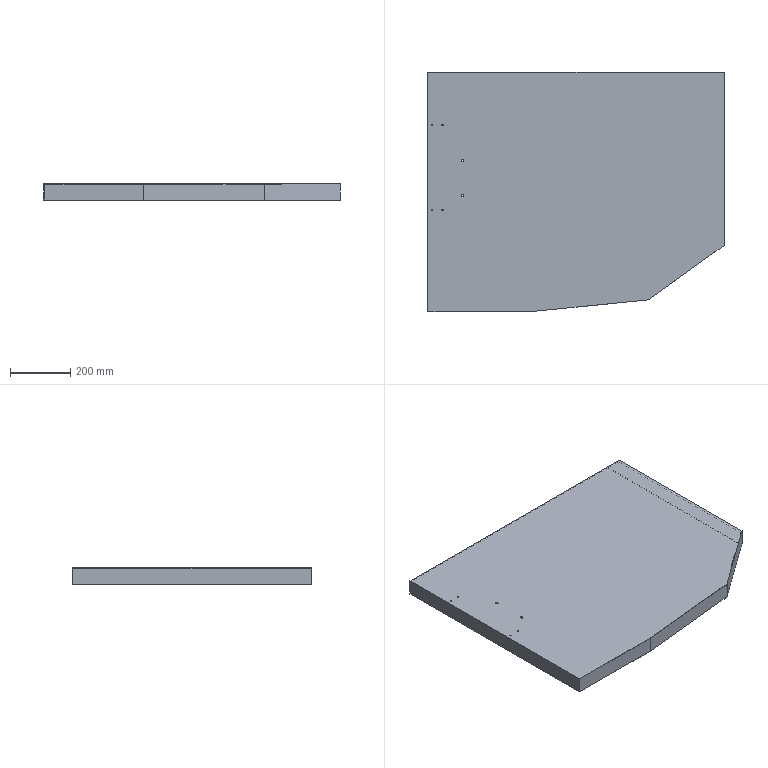Part | SolidWorks | features HoleWzd 2, ICE 2, BossThin 1, Cut 1, ExtruThin 1 | 1 solid | 41 faces | box 980 x 794 x 53 mm | volume 2935237 mm3 | plane 21 | cylinder 20 | commonest cylinder face diameters 4.2 x8 6.8 x8 8.2 x4
STEP:
#1=CARTESIAN_POINT('',(-417.615,-81.,50.));
#2=VERTEX_POINT('',#1);
#3=CARTESIAN_POINT('',(-413.415,-81.,50.));
#4=VERTEX_POINT('',#3);
#5=CARTESIAN_POINT('',(-415.515,-81.,50.));
#6=DIRECTION('',(0.,0.,1.));
#7=DIRECTION('',(1.,0.,0.));
#8=AXIS2_PLACEMENT_3D('',#5,#6,#7);
#9=CIRCLE('',#8,2.1);
#10=EDGE_CURVE('',#2,#4,#9,.T.);
#11=ORIENTED_EDGE('',*,*,#10,.F.);
#12=CARTESIAN_POINT('',(-417.615,-81.,53.));
#13=VERTEX_POINT('',#12);
#14=CARTESIAN_POINT('',(-417.615,-81.,53.));
#15=DIRECTION('',(0.,0.,1.));
#16=VECTOR('',#15,1000.);
#17=LINE('',#14,#16);
#18=EDGE_CURVE('',#2,#13,#17,.T.);
#19=ORIENTED_EDGE('',*,*,#18,.T.);
#20=CARTESIAN_POINT('',(-413.415,-81.,53.));
#21=VERTEX_POINT('',#20);
#22=CARTESIAN_POINT('',(-415.515,-81.,53.));
#23=DIRECTION('',(0.,0.,1.));
#24=DIRECTION('',(1.,0.,0.));
#25=AXIS2_PLACEMENT_3D('',#22,#23,#24);
#26=CIRCLE('',#25,2.1);
#27=EDGE_CURVE('',#13,#21,#26,.T.);
#28=ORIENTED_EDGE('',*,*,#27,.T.);
#29=CARTESIAN_POINT('',(-413.415,-81.,53.));
#30=DIRECTION('',(0.,0.,1.));
#31=VECTOR('',#30,1000.);
#32=LINE('',#29,#31);
#33=EDGE_CURVE('',#4,#21,#32,.T.);
#34=ORIENTED_EDGE('',*,*,#33,.F.);
#35=EDGE_LOOP('',(#11,#19,#28,#34));
#36=FACE_OUTER_BOUND('',#35,.T.);
#37=CARTESIAN_POINT('',(-415.515,-81.,53.));
#38=DIRECTION('',(0.,0.,1.));
#39=DIRECTION('',(1.,0.,0.));
#40=AXIS2_PLACEMENT_3D('',#37,#38,#39);
#41=CYLINDRICAL_SURFACE('',#40,2.1);
#42=ADVANCED_FACE('',(#36),#41,.F.);
#43=CARTESIAN_POINT('',(-384.115,-81.,50.));
#44=VERTEX_POINT('',#43);
#45=CARTESIAN_POINT('',(-379.915,-81.,50.));
#46=VERTEX_POINT('',#45);
#47=CARTESIAN_POINT('',(-382.015,-81.,50.));
#48=DIRECTION('',(0.,0.,1.));
#49=DIRECTION('',(1.,0.,0.));
#50=AXIS2_PLACEMENT_3D('',#47,#48,#49);
#51=CIRCLE('',#50,2.1);
#52=EDGE_CURVE('',#44,#46,#51,.T.);
#53=ORIENTED_EDGE('',*,*,#52,.F.);
#54=CARTESIAN_POINT('',(-384.115,-81.,53.));
#55=VERTEX_POINT('',#54);
#56=CARTESIAN_POINT('',(-384.115,-81.,53.));
#57=DIRECTION('',(0.,0.,1.));
#58=VECTOR('',#57,1000.);
#59=LINE('',#56,#58);
#60=EDGE_CURVE('',#44,#55,#59,.T.);
#61=ORIENTED_EDGE('',*,*,#60,.T.);
#62=CARTESIAN_POINT('',(-379.915,-81.,53.));
#63=VERTEX_POINT('',#62);
#64=CARTESIAN_POINT('',(-382.015,-81.,53.));
#65=DIRECTION('',(0.,0.,1.));
#66=DIRECTION('',(1.,0.,0.));
#67=AXIS2_PLACEMENT_3D('',#64,#65,#66);
#68=CIRCLE('',#67,2.1);
#69=EDGE_CURVE('',#55,#63,#68,.T.);
#70=ORIENTED_EDGE('',*,*,#69,.T.);
#71=CARTESIAN_POINT('',(-379.915,-81.,53.));
#72=DIRECTION('',(0.,0.,1.));
#73=VECTOR('',#72,1000.);
#74=LINE('',#71,#73);
#75=EDGE_CURVE('',#46,#63,#74,.T.);
#76=ORIENTED_EDGE('',*,*,#75,.F.);
#77=EDGE_LOOP('',(#53,#61,#70,#76));
#78=FACE_OUTER_BOUND('',#77,.T.);
#79=CARTESIAN_POINT('',(-382.015,-81.,53.));
#80=DIRECTION('',(0.,0.,1.));
#81=DIRECTION('',(1.,0.,0.));
#82=AXIS2_PLACEMENT_3D('',#79,#80,#81);
#83=CYLINDRICAL_SURFACE('',#82,2.1);
#84=ADVANCED_FACE('',(#78),#83,.F.);
#85=CARTESIAN_POINT('',(-417.615,199.,50.));
#86=VERTEX_POINT('',#85);
#87=CARTESIAN_POINT('',(-413.415,199.,50.));
#88=VERTEX_POINT('',#87);
#89=CARTESIAN_POINT('',(-415.515,199.,50.));
#90=DIRECTION('',(0.,0.,1.));
#91=DIRECTION('',(1.,0.,0.));
#92=AXIS2_PLACEMENT_3D('',#89,#90,#91);
#93=CIRCLE('',#92,2.1);
#94=EDGE_CURVE('',#86,#88,#93,.T.);
#95=ORIENTED_EDGE('',*,*,#94,.F.);
#96=CARTESIAN_POINT('',(-417.615,199.,53.));
#97=VERTEX_POINT('',#96);
#98=CARTESIAN_POINT('',(-417.615,199.,53.));
#99=DIRECTION('',(0.,0.,1.));
#100=VECTOR('',#99,1000.);
#101=LINE('',#98,#100);
#102=EDGE_CURVE('',#86,#97,#101,.T.);
#103=ORIENTED_EDGE('',*,*,#102,.T.);
#104=CARTESIAN_POINT('',(-413.415,199.,53.));
#105=VERTEX_POINT('',#104);
#106=CARTESIAN_POINT('',(-415.515,199.,53.));
#107=DIRECTION('',(0.,0.,1.));
#108=DIRECTION('',(1.,0.,0.));
#109=AXIS2_PLACEMENT_3D('',#106,#107,#108);
#110=CIRCLE('',#109,2.1);
#111=EDGE_CURVE('',#97,#105,#110,.T.);
#112=ORIENTED_EDGE('',*,*,#111,.T.);
#113=CARTESIAN_POINT('',(-413.415,199.,53.));
#114=DIRECTION('',(0.,0.,1.));
#115=VECTOR('',#114,1000.);
#116=LINE('',#113,#115);
#117=EDGE_CURVE('',#88,#105,#116,.T.);
#118=ORIENTED_EDGE('',*,*,#117,.F.);
#119=EDGE_LOOP('',(#95,#103,#112,#118));
#120=FACE_OUTER_BOUND('',#119,.T.);
#121=CARTESIAN_POINT('',(-415.515,199.,53.));
#122=DIRECTION('',(0.,0.,1.));
#123=DIRECTION('',(1.,0.,0.));
#124=AXIS2_PLACEMENT_3D('',#121,#122,#123);
#125=CYLINDRICAL_SURFACE('',#124,2.1);
#126=ADVANCED_FACE('',(#120),#125,.F.);
#127=CARTESIAN_POINT('',(-384.115,199.,50.));
#128=VERTEX_POINT('',#127);
#129=CARTESIAN_POINT('',(-379.915,199.,50.));
#130=VERTEX_POINT('',#129);
#131=CARTESIAN_POINT('',(-382.015,199.,50.));
#132=DIRECTION('',(0.,0.,1.));
#133=DIRECTION('',(1.,0.,0.));
#134=AXIS2_PLACEMENT_3D('',#131,#132,#133);
#135=CIRCLE('',#134,2.1);
#136=EDGE_CURVE('',#128,#130,#135,.T.);
#137=ORIENTED_EDGE('',*,*,#136,.F.);
#138=CARTESIAN_POINT('',(-384.115,199.,53.));
#139=VERTEX_POINT('',#138);
#140=CARTESIAN_POINT('',(-384.115,199.,53.));
#141=DIRECTION('',(0.,0.,1.));
#142=VECTOR('',#141,1000.);
#143=LINE('',#140,#142);
#144=EDGE_CURVE('',#128,#139,#143,.T.);
#145=ORIENTED_EDGE('',*,*,#144,.T.);
#146=CARTESIAN_POINT('',(-379.915,199.,53.));
#147=VERTEX_POINT('',#146);
#148=CARTESIAN_POINT('',(-382.015,199.,53.));
#149=DIRECTION('',(0.,0.,1.));
#150=DIRECTION('',(1.,0.,0.));
#151=AXIS2_PLACEMENT_3D('',#148,#149,#150);
#152=CIRCLE('',#151,2.1);
#153=EDGE_CURVE('',#139,#147,#152,.T.);
#154=ORIENTED_EDGE('',*,*,#153,.T.);
#155=CARTESIAN_POINT('',(-379.915,199.,53.));
#156=DIRECTION('',(0.,0.,1.));
#157=VECTOR('',#156,1000.);
#158=LINE('',#155,#157);
#159=EDGE_CURVE('',#130,#147,#158,.T.);
#160=ORIENTED_EDGE('',*,*,#159,.F.);
#161=EDGE_LOOP('',(#137,#145,#154,#160));
#162=FACE_OUTER_BOUND('',#161,.T.);
#163=CARTESIAN_POINT('',(-382.015,199.,53.));
#164=DIRECTION('',(0.,0.,1.));
#165=DIRECTION('',(1.,0.,0.));
#166=AXIS2_PLACEMENT_3D('',#163,#164,#165);
#167=CYLINDRICAL_SURFACE('',#166,2.1);
#168=ADVANCED_FACE('',(#162),#167,.F.);
#169=CARTESIAN_POINT('',(542.,315.,24.4));
#170=VERTEX_POINT('',#169);
#171=CARTESIAN_POINT('',(542.,315.,17.6));
#172=VERTEX_POINT('',#171);
#173=CARTESIAN_POINT('',(542.,315.,21.));
#174=DIRECTION('',(1.,0.,0.));
#175=DIRECTION('',(0.,0.,-1.));
#176=AXIS2_PLACEMENT_3D('',#173,#174,#175);
#177=CIRCLE('',#176,3.4);
#178=EDGE_CURVE('',#170,#172,#177,.T.);
#179=ORIENTED_EDGE('',*,*,#178,.F.);
#180=CARTESIAN_POINT('',(550.,315.,24.4));
#181=VERTEX_POINT('',#180);
#182=CARTESIAN_POINT('',(550.,315.,24.4));
#183=DIRECTION('',(1.,0.,0.));
#184=VECTOR('',#183,1000.);
#185=LINE('',#182,#184);
#186=EDGE_CURVE('',#170,#181,#185,.T.);
#187=ORIENTED_EDGE('',*,*,#186,.T.);
#188=CARTESIAN_POINT('',(550.,315.,17.6));
#189=VERTEX_POINT('',#188);
#190=CARTESIAN_POINT('',(550.,315.,21.));
#191=DIRECTION('',(1.,0.,0.));
#192=DIRECTION('',(0.,0.,-1.));
#193=AXIS2_PLACEMENT_3D('',#190,#191,#192);
#194=CIRCLE('',#193,3.4);
#195=EDGE_CURVE('',#181,#189,#194,.T.);
#196=ORIENTED_EDGE('',*,*,#195,.T.);
#197=CARTESIAN_POINT('',(550.,315.,17.6));
#198=DIRECTION('',(1.,0.,0.));
#199=VECTOR('',#198,1000.);
#200=LINE('',#197,#199);
#201=EDGE_CURVE('',#172,#189,#200,.T.);
#202=ORIENTED_EDGE('',*,*,#201,.F.);
#203=EDGE_LOOP('',(#179,#187,#196,#202));
#204=FACE_OUTER_BOUND('',#203,.T.);
#205=CARTESIAN_POINT('',(550.,315.,21.));
#206=DIRECTION('',(1.,0.,0.));
#207=DIRECTION('',(0.,0.,-1.));
#208=AXIS2_PLACEMENT_3D('',#205,#206,#207);
#209=CYLINDRICAL_SURFACE('',#208,3.4);
#210=ADVANCED_FACE('',(#204),#209,.F.);
#211=CARTESIAN_POINT('',(542.,285.,24.4));
#212=VERTEX_POINT('',#211);
#213=CARTESIAN_POINT('',(542.,285.,17.6));
#214=VERTEX_POINT('',#213);
#215=CARTESIAN_POINT('',(542.,285.,21.));
#216=DIRECTION('',(1.,0.,0.));
#217=DIRECTION('',(0.,0.,-1.));
#218=AXIS2_PLACEMENT_3D('',#215,#216,#217);
#219=CIRCLE('',#218,3.4);
#220=EDGE_CURVE('',#212,#214,#219,.T.);
#221=ORIENTED_EDGE('',*,*,#220,.F.);
#222=CARTESIAN_POINT('',(550.,285.,24.4));
#223=VERTEX_POINT('',#222);
#224=CARTESIAN_POINT('',(550.,285.,24.4));
#225=DIRECTION('',(1.,0.,0.));
#226=VECTOR('',#225,1000.);
#227=LINE('',#224,#226);
#228=EDGE_CURVE('',#212,#223,#227,.T.);
#229=ORIENTED_EDGE('',*,*,#228,.T.);
#230=CARTESIAN_POINT('',(550.,285.,17.6));
#231=VERTEX_POINT('',#230);
#232=CARTESIAN_POINT('',(550.,285.,21.));
#233=DIRECTION('',(1.,0.,0.));
#234=DIRECTION('',(0.,0.,-1.));
#235=AXIS2_PLACEMENT_3D('',#232,#233,#234);
#236=CIRCLE('',#235,3.4);
#237=EDGE_CURVE('',#223,#231,#236,.T.);
#238=ORIENTED_EDGE('',*,*,#237,.T.);
#239=CARTESIAN_POINT('',(550.,285.,17.6));
#240=DIRECTION('',(1.,0.,0.));
#241=VECTOR('',#240,1000.);
#242=LINE('',#239,#241);
#243=EDGE_CURVE('',#214,#231,#242,.T.);
#244=ORIENTED_EDGE('',*,*,#243,.F.);
#245=EDGE_LOOP('',(#221,#229,#238,#244));
#246=FACE_OUTER_BOUND('',#245,.T.);
#247=CARTESIAN_POINT('',(550.,285.,21.));
#248=DIRECTION('',(1.,0.,0.));
#249=DIRECTION('',(0.,0.,-1.));
#250=AXIS2_PLACEMENT_3D('',#247,#248,#249);
#251=CYLINDRICAL_SURFACE('',#250,3.4);
#252=ADVANCED_FACE('',(#246),#251,.F.);
#253=CARTESIAN_POINT('',(542.,45.,24.4));
#254=VERTEX_POINT('',#253);
#255=CARTESIAN_POINT('',(542.,45.,17.6));
#256=VERTEX_POINT('',#255);
#257=CARTESIAN_POINT('',(542.,45.,21.));
#258=DIRECTION('',(1.,0.,0.));
#259=DIRECTION('',(0.,0.,-1.));
#260=AXIS2_PLACEMENT_3D('',#257,#258,#259);
#261=CIRCLE('',#260,3.4);
#262=EDGE_CURVE('',#254,#256,#261,.T.);
#263=ORIENTED_EDGE('',*,*,#262,.F.);
#264=CARTESIAN_POINT('',(550.,45.,24.4));
#265=VERTEX_POINT('',#264);
#266=CARTESIAN_POINT('',(550.,45.,24.4));
#267=DIRECTION('',(1.,0.,0.));
#268=VECTOR('',#267,1000.);
#269=LINE('',#266,#268);
#270=EDGE_CURVE('',#254,#265,#269,.T.);
#271=ORIENTED_EDGE('',*,*,#270,.T.);
#272=CARTESIAN_POINT('',(550.,45.,17.6));
#273=VERTEX_POINT('',#272);
#274=CARTESIAN_POINT('',(550.,45.,21.));
#275=DIRECTION('',(1.,0.,0.));
#276=DIRECTION('',(0.,0.,-1.));
#277=AXIS2_PLACEMENT_3D('',#274,#275,#276);
#278=CIRCLE('',#277,3.4);
#279=EDGE_CURVE('',#265,#273,#278,.T.);
#280=ORIENTED_EDGE('',*,*,#279,.T.);
#281=CARTESIAN_POINT('',(550.,45.,17.6));
#282=DIRECTION('',(1.,0.,0.));
#283=VECTOR('',#282,1000.);
#284=LINE('',#281,#283);
#285=EDGE_CURVE('',#256,#273,#284,.T.);
#286=ORIENTED_EDGE('',*,*,#285,.F.);
#287=EDGE_LOOP('',(#263,#271,#280,#286));
#288=FACE_OUTER_BOUND('',#287,.T.);
#289=CARTESIAN_POINT('',(550.,45.,21.));
#290=DIRECTION('',(1.,0.,0.));
#291=DIRECTION('',(0.,0.,-1.));
#292=AXIS2_PLACEMENT_3D('',#289,#290,#291);
#293=CYLINDRICAL_SURFACE('',#292,3.4);
#294=ADVANCED_FACE('',(#288),#293,.F.);
#295=CARTESIAN_POINT('',(-312.4,82.25,50.));
#296=VERTEX_POINT('',#295);
#297=CARTESIAN_POINT('',(-320.6,82.25,50.));
#298=VERTEX_POINT('',#297);
#299=CARTESIAN_POINT('',(-316.5,82.25,50.));
#300=DIRECTION('',(0.,0.,-1.));
#301=DIRECTION('',(1.,0.,0.));
#302=AXIS2_PLACEMENT_3D('',#299,#300,#301);
#303=CIRCLE('',#302,4.1);
#304=EDGE_CURVE('',#296,#298,#303,.T.);
#305=ORIENTED_EDGE('',*,*,#304,.T.);
#306=CARTESIAN_POINT('',(-320.6,82.25,53.));
#307=VERTEX_POINT('',#306);
#308=CARTESIAN_POINT('',(-320.6,82.25,-0.001));
#309=DIRECTION('',(0.,0.,1.));
#310=VECTOR('',#309,1000.);
#311=LINE('',#308,#310);
#312=EDGE_CURVE('',#298,#307,#311,.T.);
#313=ORIENTED_EDGE('',*,*,#312,.T.);
#314=CARTESIAN_POINT('',(-312.4,82.25,53.));
#315=VERTEX_POINT('',#314);
#316=CARTESIAN_POINT('',(-316.5,82.25,53.));
#317=DIRECTION('',(0.,0.,1.));
#318=DIRECTION('',(1.,0.,0.));
#319=AXIS2_PLACEMENT_3D('',#316,#317,#318);
#320=CIRCLE('',#319,4.1);
#321=EDGE_CURVE('',#307,#315,#320,.T.);
#322=ORIENTED_EDGE('',*,*,#321,.T.);
#323=CARTESIAN_POINT('',(-312.4,82.25,-0.001));
#324=DIRECTION('',(0.,0.,1.));
#325=VECTOR('',#324,1000.);
#326=LINE('',#323,#325);
#327=EDGE_CURVE('',#296,#315,#326,.T.);
#328=ORIENTED_EDGE('',*,*,#327,.F.);
#329=EDGE_LOOP('',(#305,#313,#322,#328));
#330=FACE_OUTER_BOUND('',#329,.T.);
#331=CARTESIAN_POINT('',(-316.5,82.25,-0.001));
#332=DIRECTION('',(0.,0.,1.));
#333=DIRECTION('',(1.,0.,0.));
#334=AXIS2_PLACEMENT_3D('',#331,#332,#333);
#335=CYLINDRICAL_SURFACE('',#334,4.1);
#336=ADVANCED_FACE('',(#330),#335,.F.);
#337=CARTESIAN_POINT('',(-312.4,-34.25,50.));
#338=VERTEX_POINT('',#337);
#339=CARTESIAN_POINT('',(-320.6,-34.25,50.));
#340=VERTEX_POINT('',#339);
#341=CARTESIAN_POINT('',(-316.5,-34.25,50.));
#342=DIRECTION('',(0.,0.,-1.));
#343=DIRECTION('',(1.,0.,0.));
#344=AXIS2_PLACEMENT_3D('',#341,#342,#343);
#345=CIRCLE('',#344,4.1);
#346=EDGE_CURVE('',#338,#340,#345,.T.);
#347=ORIENTED_EDGE('',*,*,#346,.T.);
#348=CARTESIAN_POINT('',(-320.6,-34.25,53.));
#349=VERTEX_POINT('',#348);
#350=CARTESIAN_POINT('',(-320.6,-34.25,-0.001));
#351=DIRECTION('',(0.,0.,1.));
#352=VECTOR('',#351,1000.);
#353=LINE('',#350,#352);
#354=EDGE_CURVE('',#340,#349,#353,.T.);
#355=ORIENTED_EDGE('',*,*,#354,.T.);
#356=CARTESIAN_POINT('',(-312.4,-34.25,53.));
#357=VERTEX_POINT('',#356);
#358=CARTESIAN_POINT('',(-316.5,-34.25,53.));
#359=DIRECTION('',(0.,0.,1.));
#360=DIRECTION('',(1.,0.,0.));
#361=AXIS2_PLACEMENT_3D('',#358,#359,#360);
#362=CIRCLE('',#361,4.1);
#363=EDGE_CURVE('',#349,#357,#362,.T.);
#364=ORIENTED_EDGE('',*,*,#363,.T.);
#365=CARTESIAN_POINT('',(-312.4,-34.25,-0.001));
#366=DIRECTION('',(0.,0.,1.));
#367=VECTOR('',#366,1000.);
#368=LINE('',#365,#367);
#369=EDGE_CURVE('',#338,#357,#368,.T.);
#370=ORIENTED_EDGE('',*,*,#369,.F.);
#371=EDGE_LOOP('',(#347,#355,#364,#370));
#372=FACE_OUTER_BOUND('',#371,.T.);
#373=CARTESIAN_POINT('',(-316.5,-34.25,-0.001));
#374=DIRECTION('',(0.,0.,1.));
#375=DIRECTION('',(1.,0.,0.));
#376=AXIS2_PLACEMENT_3D('',#373,#374,#375);
#377=CYLINDRICAL_SURFACE('',#376,4.1);
#378=ADVANCED_FACE('',(#372),#377,.F.);
#379=CARTESIAN_POINT('',(542.,15.,24.4));
#380=VERTEX_POINT('',#379);
#381=CARTESIAN_POINT('',(542.,15.,17.6));
#382=VERTEX_POINT('',#381);
#383=CARTESIAN_POINT('',(542.,15.,21.));
#384=DIRECTION('',(1.,0.,0.));
#385=DIRECTION('',(0.,0.,-1.));
#386=AXIS2_PLACEMENT_3D('',#383,#384,#385);
#387=CIRCLE('',#386,3.4);
#388=EDGE_CURVE('',#380,#382,#387,.T.);
#389=ORIENTED_EDGE('',*,*,#388,.F.);
#390=CARTESIAN_POINT('',(550.,15.,24.4));
#391=VERTEX_POINT('',#390);
#392=CARTESIAN_POINT('',(550.,15.,24.4));
#393=DIRECTION('',(1.,0.,0.));
#394=VECTOR('',#393,1000.);
#395=LINE('',#392,#394);
#396=EDGE_CURVE('',#380,#391,#395,.T.);
#397=ORIENTED_EDGE('',*,*,#396,.T.);
#398=CARTESIAN_POINT('',(550.,15.,17.6));
#399=VERTEX_POINT('',#398);
#400=CARTESIAN_POINT('',(550.,15.,21.));
#401=DIRECTION('',(1.,0.,0.));
#402=DIRECTION('',(0.,0.,-1.));
#403=AXIS2_PLACEMENT_3D('',#400,#401,#402);
#404=CIRCLE('',#403,3.4);
#405=EDGE_CURVE('',#391,#399,#404,.T.);
#406=ORIENTED_EDGE('',*,*,#405,.T.);
#407=CARTESIAN_POINT('',(550.,15.,17.6));
#408=DIRECTION('',(1.,0.,0.));
#409=VECTOR('',#408,1000.);
#410=LINE('',#407,#409);
#411=EDGE_CURVE('',#382,#399,#410,.T.);
#412=ORIENTED_EDGE('',*,*,#411,.F.);
#413=EDGE_LOOP('',(#389,#397,#406,#412));
#414=FACE_OUTER_BOUND('',#413,.T.);
#415=CARTESIAN_POINT('',(550.,15.,21.));
#416=DIRECTION('',(1.,0.,0.));
#417=DIRECTION('',(0.,0.,-1.));
#418=AXIS2_PLACEMENT_3D('',#415,#416,#417);
#419=CYLINDRICAL_SURFACE('',#418,3.4);
#420=ADVANCED_FACE('',(#414),#419,.F.);
#421=CARTESIAN_POINT('',(550.,-199.,53.));
#422=VERTEX_POINT('',#421);
#423=CARTESIAN_POINT('',(550.,-199.,0.));
#424=VERTEX_POINT('',#423);
#425=CARTESIAN_POINT('',(550.,-199.,53.));
#426=DIRECTION('',(0.,0.,-1.));
#427=VECTOR('',#426,1000.);
#428=LINE('',#425,#427);
#429=EDGE_CURVE('',#422,#424,#428,.T.);
#430=ORIENTED_EDGE('',*,*,#429,.T.);
#431=CARTESIAN_POINT('',(550.,375.,0.));
#432=VERTEX_POINT('',#431);
#433=CARTESIAN_POINT('',(550.,375.,0.));
#434=DIRECTION('',(0.,1.,0.));
#435=VECTOR('',#434,1000.);
#436=LINE('',#433,#435);
#437=EDGE_CURVE('',#424,#432,#436,.T.);
#438=ORIENTED_EDGE('',*,*,#437,.T.);
#439=CARTESIAN_POINT('',(550.,375.,53.));
#440=VERTEX_POINT('',#439);
#441=CARTESIAN_POINT('',(550.,375.,53.));
#442=DIRECTION('',(0.,0.,-1.));
#443=VECTOR('',#442,1000.);
#444=LINE('',#441,#443);
#445=EDGE_CURVE('',#440,#432,#444,.T.);
#446=ORIENTED_EDGE('',*,*,#445,.F.);
#447=CARTESIAN_POINT('',(550.,375.,53.));
#448=DIRECTION('',(0.,1.,0.));
#449=VECTOR('',#448,1000.);
#450=LINE('',#447,#449);
#451=EDGE_CURVE('',#422,#440,#450,.T.);
#452=ORIENTED_EDGE('',*,*,#451,.F.);
#453=EDGE_LOOP('',(#430,#438,#446,#452));
#454=FACE_OUTER_BOUND('',#453,.T.);
#455=CARTESIAN_POINT('',(550.,15.,21.));
#456=DIRECTION('',(1.,0.,0.));
#457=DIRECTION('',(0.,0.,-1.));
#458=AXIS2_PLACEMENT_3D('',#455,#456,#457);
#459=CIRCLE('',#458,3.4);
#460=EDGE_CURVE('',#399,#391,#459,.T.);
#461=ORIENTED_EDGE('',*,*,#460,.F.);
#462=ORIENTED_EDGE('',*,*,#405,.F.);
#463=EDGE_LOOP('',(#461,#462));
#464=FACE_BOUND('',#463,.T.);
#465=CARTESIAN_POINT('',(550.,45.,21.));
#466=DIRECTION('',(1.,0.,0.));
#467=DIRECTION('',(0.,0.,-1.));
#468=AXIS2_PLACEMENT_3D('',#465,#466,#467);
#469=CIRCLE('',#468,3.4);
#470=EDGE_CURVE('',#273,#265,#469,.T.);
#471=ORIENTED_EDGE('',*,*,#470,.F.);
#472=ORIENTED_EDGE('',*,*,#279,.F.);
#473=EDGE_LOOP('',(#471,#472));
#474=FACE_BOUND('',#473,.T.);
#475=CARTESIAN_POINT('',(550.,285.,21.));
#476=DIRECTION('',(1.,0.,0.));
#477=DIRECTION('',(0.,0.,-1.));
#478=AXIS2_PLACEMENT_3D('',#475,#476,#477);
#479=CIRCLE('',#478,3.4);
#480=EDGE_CURVE('',#231,#223,#479,.T.);
#481=ORIENTED_EDGE('',*,*,#480,.F.);
#482=ORIENTED_EDGE('',*,*,#237,.F.);
#483=EDGE_LOOP('',(#481,#482));
#484=FACE_BOUND('',#483,.T.);
#485=CARTESIAN_POINT('',(550.,315.,21.));
#486=DIRECTION('',(1.,0.,0.));
#487=DIRECTION('',(0.,0.,-1.));
#488=AXIS2_PLACEMENT_3D('',#485,#486,#487);
#489=CIRCLE('',#488,3.4);
#490=EDGE_CURVE('',#189,#181,#489,.T.);
#491=ORIENTED_EDGE('',*,*,#490,.F.);
#492=ORIENTED_EDGE('',*,*,#195,.F.);
#493=EDGE_LOOP('',(#491,#492));
#494=FACE_BOUND('',#493,.T.);
#495=CARTESIAN_POINT('',(550.,375.,53.));
#496=DIRECTION('',(-1.,0.,0.));
#497=DIRECTION('',(0.,-1.,0.));
#498=AXIS2_PLACEMENT_3D('',#495,#496,#497);
#499=PLANE('',#498);
#500=ADVANCED_FACE('',(#454,#464,#474,#484,#494),#499,.F.);
#501=CARTESIAN_POINT('',(542.,315.,21.));
#502=DIRECTION('',(1.,0.,0.));
#503=DIRECTION('',(0.,0.,-1.));
#504=AXIS2_PLACEMENT_3D('',#501,#502,#503);
#505=CIRCLE('',#504,3.4);
#506=EDGE_CURVE('',#172,#170,#505,.T.);
#507=ORIENTED_EDGE('',*,*,#506,.T.);
#508=ORIENTED_EDGE('',*,*,#178,.T.);
#509=EDGE_LOOP('',(#507,#508));
#510=FACE_BOUND('',#509,.T.);
#511=CARTESIAN_POINT('',(542.,285.,21.));
#512=DIRECTION('',(1.,0.,0.));
#513=DIRECTION('',(0.,0.,-1.));
#514=AXIS2_PLACEMENT_3D('',#511,#512,#513);
#515=CIRCLE('',#514,3.4);
#516=EDGE_CURVE('',#214,#212,#515,.T.);
#517=ORIENTED_EDGE('',*,*,#516,.T.);
#518=ORIENTED_EDGE('',*,*,#220,.T.);
#519=EDGE_LOOP('',(#517,#518));
#520=FACE_BOUND('',#519,.T.);
#521=CARTESIAN_POINT('',(542.,45.,21.));
#522=DIRECTION('',(1.,0.,0.));
#523=DIRECTION('',(0.,0.,-1.));
#524=AXIS2_PLACEMENT_3D('',#521,#522,#523);
#525=CIRCLE('',#524,3.4);
#526=EDGE_CURVE('',#256,#254,#525,.T.);
#527=ORIENTED_EDGE('',*,*,#526,.T.);
#528=ORIENTED_EDGE('',*,*,#262,.T.);
#529=EDGE_LOOP('',(#527,#528));
#530=FACE_BOUND('',#529,.T.);
#531=CARTESIAN_POINT('',(542.,15.,21.));
#532=DIRECTION('',(1.,0.,0.));
#533=DIRECTION('',(0.,0.,-1.));
#534=AXIS2_PLACEMENT_3D('',#531,#532,#533);
#535=CIRCLE('',#534,3.4);
#536=EDGE_CURVE('',#382,#380,#535,.T.);
#537=ORIENTED_EDGE('',*,*,#536,.T.);
#538=ORIENTED_EDGE('',*,*,#388,.T.);
#539=EDGE_LOOP('',(#537,#538));
#540=FACE_BOUND('',#539,.T.);
#541=CARTESIAN_POINT('',(542.,372.,10.612));
#542=VERTEX_POINT('',#541);
#543=CARTESIAN_POINT('',(542.,372.,50.));
#544=VERTEX_POINT('',#543);
#545=CARTESIAN_POINT('',(542.,372.,53.));
#546=DIRECTION('',(0.,0.,1.));
#547=VECTOR('',#546,1000.);
#548=LINE('',#545,#547);
#549=EDGE_CURVE('',#542,#544,#548,.T.);
#550=ORIENTED_EDGE('',*,*,#549,.F.);
#551=CARTESIAN_POINT('',(542.,-201.063,10.612));
#552=VERTEX_POINT('',#551);
#553=CARTESIAN_POINT('',(542.,-201.063,10.612));
#554=DIRECTION('',(0.,-1.,0.));
#555=VECTOR('',#554,1000.);
#556=LINE('',#553,#555);
#557=EDGE_CURVE('',#542,#552,#556,.T.);
#558=ORIENTED_EDGE('',*,*,#557,.T.);
#559=CARTESIAN_POINT('',(542.,-201.063,50.));
#560=VERTEX_POINT('',#559);
#561=CARTESIAN_POINT('',(542.,-201.063,-576.119));
#562=DIRECTION('',(0.,0.,1.));
#563=VECTOR('',#562,1000.);
#564=LINE('',#561,#563);
#565=EDGE_CURVE('',#552,#560,#564,.T.);
#566=ORIENTED_EDGE('',*,*,#565,.T.);
#567=CARTESIAN_POINT('',(542.,-201.063,50.));
#568=DIRECTION('',(0.,1.,0.));
#569=VECTOR('',#568,1000.);
#570=LINE('',#567,#569);
#571=EDGE_CURVE('',#560,#544,#570,.T.);
#572=ORIENTED_EDGE('',*,*,#571,.T.);
#573=EDGE_LOOP('',(#550,#558,#566,#572));
#574=FACE_OUTER_BOUND('',#573,.T.);
#575=CARTESIAN_POINT('',(542.,-201.063,-576.119));
#576=DIRECTION('',(1.,0.,0.));
#577=DIRECTION('',(0.,0.,-1.));
#578=AXIS2_PLACEMENT_3D('',#575,#576,#577);
#579=PLANE('',#578);
#580=ADVANCED_FACE('',(#510,#520,#530,#540,#574),#579,.F.);
#581=CARTESIAN_POINT('',(495.109,-234.824,50.));
#582=VERTEX_POINT('',#581);
#583=CARTESIAN_POINT('',(280.386,-389.425,50.));
#584=DIRECTION('',(0.8115,0.5843,0.));
#585=VECTOR('',#584,1000.);
#586=LINE('',#583,#585);
#587=EDGE_CURVE('',#582,#560,#586,.T.);
#588=ORIENTED_EDGE('',*,*,#587,.F.);
#589=CARTESIAN_POINT('',(495.109,372.,50.));
#590=VERTEX_POINT('',#589);
#591=CARTESIAN_POINT('',(495.109,0.,50.));
#592=DIRECTION('',(0.,1.,0.));
#593=VECTOR('',#592,1000.);
#594=LINE('',#591,#593);
#595=EDGE_CURVE('',#582,#590,#594,.T.);
#596=ORIENTED_EDGE('',*,*,#595,.T.);
#597=CARTESIAN_POINT('',(0.,372.,50.));
#598=DIRECTION('',(-1.,0.,0.));
#599=VECTOR('',#598,1000.);
#600=LINE('',#597,#599);
#601=EDGE_CURVE('',#544,#590,#600,.T.);
#602=ORIENTED_EDGE('',*,*,#601,.F.);
#603=ORIENTED_EDGE('',*,*,#571,.F.);
#604=EDGE_LOOP('',(#588,#596,#602,#603));
#605=FACE_OUTER_BOUND('',#604,.T.);
#606=CARTESIAN_POINT('',(0.,0.,50.));
#607=DIRECTION('',(0.,0.,1.));
#608=DIRECTION('',(1.,0.,0.));
#609=AXIS2_PLACEMENT_3D('',#606,#607,#608);
#610=PLANE('',#609);
#611=ADVANCED_FACE('',(#605),#610,.F.);
#612=CARTESIAN_POINT('',(474.657,-249.55,67.18));
#613=DIRECTION('',(-0.6706,-0.4828,0.5633));
#614=VECTOR('',#613,1000.);
#615=LINE('',#612,#614);
#616=EDGE_CURVE('',#552,#582,#615,.T.);
#617=ORIENTED_EDGE('',*,*,#616,.T.);
#618=ORIENTED_EDGE('',*,*,#587,.T.);
#619=ORIENTED_EDGE('',*,*,#565,.F.);
#620=EDGE_LOOP('',(#617,#618,#619));
#621=FACE_OUTER_BOUND('',#620,.T.);
#622=CARTESIAN_POINT('',(280.386,-389.425,53.));
#623=DIRECTION('',(-0.5843,0.8115,0.));
#624=DIRECTION('',(-0.8115,-0.5843,0.));
#625=AXIS2_PLACEMENT_3D('',#622,#623,#624);
#626=PLANE('',#625);
#627=ADVANCED_FACE('',(#621),#626,.T.);
#628=CARTESIAN_POINT('',(493.286,372.,51.531));
#629=DIRECTION('',(0.7657,0.,-0.6432));
#630=VECTOR('',#629,1000.);
#631=LINE('',#628,#630);
#632=EDGE_CURVE('',#590,#542,#631,.T.);
#633=ORIENTED_EDGE('',*,*,#632,.T.);
#634=ORIENTED_EDGE('',*,*,#549,.T.);
#635=ORIENTED_EDGE('',*,*,#601,.T.);
#636=EDGE_LOOP('',(#633,#634,#635));
#637=FACE_OUTER_BOUND('',#636,.T.);
#638=CARTESIAN_POINT('',(0.,372.,53.));
#639=DIRECTION('',(0.,-1.,0.));
#640=DIRECTION('',(1.,0.,0.));
#641=AXIS2_PLACEMENT_3D('',#638,#639,#640);
#642=PLANE('',#641);
#643=ADVANCED_FACE('',(#637),#642,.T.);
#644=ORIENTED_EDGE('',*,*,#595,.F.);
#645=ORIENTED_EDGE('',*,*,#616,.F.);
#646=ORIENTED_EDGE('',*,*,#557,.F.);
#647=ORIENTED_EDGE('',*,*,#632,.F.);
#648=EDGE_LOOP('',(#644,#645,#646,#647));
#649=FACE_OUTER_BOUND('',#648,.T.);
#650=CARTESIAN_POINT('',(493.286,-293.682,51.531));
#651=DIRECTION('',(0.6432,0.,0.7657));
#652=DIRECTION('',(0.7657,0.,-0.6432));
#653=AXIS2_PLACEMENT_3D('',#650,#651,#652);
#654=PLANE('',#653);
#655=ADVANCED_FACE('',(#649),#654,.T.);
#656=ORIENTED_EDGE('',*,*,#396,.F.);
#657=ORIENTED_EDGE('',*,*,#536,.F.);
#658=ORIENTED_EDGE('',*,*,#411,.T.);
#659=ORIENTED_EDGE('',*,*,#460,.T.);
#660=EDGE_LOOP('',(#656,#657,#658,#659));
#661=FACE_OUTER_BOUND('',#660,.T.);
#662=CARTESIAN_POINT('',(550.,15.,21.));
#663=DIRECTION('',(1.,0.,0.));
#664=DIRECTION('',(0.,0.,-1.));
#665=AXIS2_PLACEMENT_3D('',#662,#663,#664);
#666=CYLINDRICAL_SURFACE('',#665,3.4);
#667=ADVANCED_FACE('',(#661),#666,.F.);
#668=CARTESIAN_POINT('',(542.,372.,0.));
#669=VERTEX_POINT('',#668);
#670=CARTESIAN_POINT('',(542.,372.,8.));
#671=VERTEX_POINT('',#670);
#672=CARTESIAN_POINT('',(542.,372.,53.));
#673=DIRECTION('',(0.,0.,1.));
#674=VECTOR('',#673,1000.);
#675=LINE('',#672,#674);
#676=EDGE_CURVE('',#669,#671,#675,.T.);
#677=ORIENTED_EDGE('',*,*,#676,.T.);
#678=CARTESIAN_POINT('',(492.,372.,50.));
#679=VERTEX_POINT('',#678);
#680=CARTESIAN_POINT('',(492.,372.,50.));
#681=DIRECTION('',(0.7657,0.,-0.6432));
#682=VECTOR('',#681,1000.);
#683=LINE('',#680,#682);
#684=EDGE_CURVE('',#679,#671,#683,.T.);
#685=ORIENTED_EDGE('',*,*,#684,.F.);
#686=CARTESIAN_POINT('',(-427.,372.,50.));
#687=VERTEX_POINT('',#686);
#688=CARTESIAN_POINT('',(0.,372.,50.));
#689=DIRECTION('',(-1.,0.,0.));
#690=VECTOR('',#689,1000.);
#691=LINE('',#688,#690);
#692=EDGE_CURVE('',#679,#687,#691,.T.);
#693=ORIENTED_EDGE('',*,*,#692,.T.);
#694=CARTESIAN_POINT('',(-427.,372.,0.));
#695=VERTEX_POINT('',#694);
#696=CARTESIAN_POINT('',(-427.,372.,53.));
#697=DIRECTION('',(0.,0.,-1.));
#698=VECTOR('',#697,1000.);
#699=LINE('',#696,#698);
#700=EDGE_CURVE('',#687,#695,#699,.T.);
#701=ORIENTED_EDGE('',*,*,#700,.T.);
#702=CARTESIAN_POINT('',(0.,372.,0.));
#703=DIRECTION('',(-1.,0.,0.));
#704=VECTOR('',#703,1000.);
#705=LINE('',#702,#704);
#706=EDGE_CURVE('',#669,#695,#705,.T.);
#707=ORIENTED_EDGE('',*,*,#706,.F.);
#708=EDGE_LOOP('',(#677,#685,#693,#701,#707));
#709=FACE_OUTER_BOUND('',#708,.T.);
#710=CARTESIAN_POINT('',(0.,372.,53.));
#711=DIRECTION('',(0.,-1.,0.));
#712=DIRECTION('',(1.,0.,0.));
#713=AXIS2_PLACEMENT_3D('',#710,#711,#712);
#714=PLANE('',#713);
#715=ADVANCED_FACE('',(#709),#714,.T.);
#716=CARTESIAN_POINT('',(298.9,-376.095,50.));
#717=VERTEX_POINT('',#716);
#718=CARTESIAN_POINT('',(492.,-237.063,50.));
#719=VERTEX_POINT('',#718);
#720=CARTESIAN_POINT('',(280.386,-389.425,50.));
#721=DIRECTION('',(0.8115,0.5843,0.));
#722=VECTOR('',#721,1000.);
#723=LINE('',#720,#722);
#724=EDGE_CURVE('',#717,#719,#723,.T.);
#725=ORIENTED_EDGE('',*,*,#724,.T.);
#726=CARTESIAN_POINT('',(542.,-201.063,8.));
#727=VERTEX_POINT('',#726);
#728=CARTESIAN_POINT('',(473.67,-250.261,65.397));
#729=DIRECTION('',(-0.6706,-0.4828,0.5633));
#730=VECTOR('',#729,1000.);
#731=LINE('',#728,#730);
#732=EDGE_CURVE('',#727,#719,#731,.T.);
#733=ORIENTED_EDGE('',*,*,#732,.F.);
#734=CARTESIAN_POINT('',(542.,-201.063,0.));
#735=VERTEX_POINT('',#734);
#736=CARTESIAN_POINT('',(542.,-201.063,-576.119));
#737=DIRECTION('',(0.,0.,1.));
#738=VECTOR('',#737,1000.);
#739=LINE('',#736,#738);
#740=EDGE_CURVE('',#735,#727,#739,.T.);
#741=ORIENTED_EDGE('',*,*,#740,.F.);
#742=CARTESIAN_POINT('',(298.9,-376.095,0.));
#743=VERTEX_POINT('',#742);
#744=CARTESIAN_POINT('',(280.386,-389.425,0.));
#745=DIRECTION('',(0.8115,0.5843,0.));
#746=VECTOR('',#745,1000.);
#747=LINE('',#744,#746);
#748=EDGE_CURVE('',#743,#735,#747,.T.);
#749=ORIENTED_EDGE('',*,*,#748,.F.);
#750=CARTESIAN_POINT('',(298.9,-376.095,53.));
#751=DIRECTION('',(0.,0.,-1.));
#752=VECTOR('',#751,1000.);
#753=LINE('',#750,#752);
#754=EDGE_CURVE('',#717,#743,#753,.T.);
#755=ORIENTED_EDGE('',*,*,#754,.F.);
#756=EDGE_LOOP('',(#725,#733,#741,#749,#755));
#757=FACE_OUTER_BOUND('',#756,.T.);
#758=CARTESIAN_POINT('',(280.386,-389.425,53.));
#759=DIRECTION('',(-0.5843,0.8115,0.));
#760=DIRECTION('',(-0.8115,-0.5843,0.));
#761=AXIS2_PLACEMENT_3D('',#758,#759,#760);
#762=PLANE('',#761);
#763=ADVANCED_FACE('',(#757),#762,.T.);
#764=ORIENTED_EDGE('',*,*,#740,.T.);
#765=CARTESIAN_POINT('',(542.,-293.682,8.));
#766=DIRECTION('',(0.,1.,0.));
#767=VECTOR('',#766,1000.);
#768=LINE('',#765,#767);
#769=EDGE_CURVE('',#727,#671,#768,.T.);
#770=ORIENTED_EDGE('',*,*,#769,.T.);
#771=ORIENTED_EDGE('',*,*,#676,.F.);
#772=CARTESIAN_POINT('',(542.,-201.063,0.));
#773=DIRECTION('',(0.,-1.,0.));
#774=VECTOR('',#773,1000.);
#775=LINE('',#772,#774);
#776=EDGE_CURVE('',#669,#735,#775,.T.);
#777=ORIENTED_EDGE('',*,*,#776,.T.);
#778=EDGE_LOOP('',(#764,#770,#771,#777));
#779=FACE_OUTER_BOUND('',#778,.T.);
#780=CARTESIAN_POINT('',(542.,-201.063,-576.119));
#781=DIRECTION('',(1.,0.,0.));
#782=DIRECTION('',(0.,0.,-1.));
#783=AXIS2_PLACEMENT_3D('',#780,#781,#782);
#784=PLANE('',#783);
#785=ADVANCED_FACE('',(#779),#784,.F.);
#786=CARTESIAN_POINT('',(-415.515,-81.,50.));
#787=DIRECTION('',(0.,0.,1.));
#788=DIRECTION('',(1.,0.,0.));
#789=AXIS2_PLACEMENT_3D('',#786,#787,#788);
#790=CIRCLE('',#789,2.1);
#791=EDGE_CURVE('',#4,#2,#790,.T.);
#792=ORIENTED_EDGE('',*,*,#791,.T.);
#793=ORIENTED_EDGE('',*,*,#10,.T.);
#794=EDGE_LOOP('',(#792,#793));
#795=FACE_BOUND('',#794,.T.);
#796=CARTESIAN_POINT('',(-382.015,-81.,50.));
#797=DIRECTION('',(0.,0.,1.));
#798=DIRECTION('',(1.,0.,0.));
#799=AXIS2_PLACEMENT_3D('',#796,#797,#798);
#800=CIRCLE('',#799,2.1);
#801=EDGE_CURVE('',#46,#44,#800,.T.);
#802=ORIENTED_EDGE('',*,*,#801,.T.);
#803=ORIENTED_EDGE('',*,*,#52,.T.);
#804=EDGE_LOOP('',(#802,#803));
#805=FACE_BOUND('',#804,.T.);
#806=CARTESIAN_POINT('',(-415.515,199.,50.));
#807=DIRECTION('',(0.,0.,1.));
#808=DIRECTION('',(1.,0.,0.));
#809=AXIS2_PLACEMENT_3D('',#806,#807,#808);
#810=CIRCLE('',#809,2.1);
#811=EDGE_CURVE('',#88,#86,#810,.T.);
#812=ORIENTED_EDGE('',*,*,#811,.T.);
#813=ORIENTED_EDGE('',*,*,#94,.T.);
#814=EDGE_LOOP('',(#812,#813));
#815=FACE_BOUND('',#814,.T.);
#816=CARTESIAN_POINT('',(-382.015,199.,50.));
#817=DIRECTION('',(0.,0.,1.));
#818=DIRECTION('',(1.,0.,0.));
#819=AXIS2_PLACEMENT_3D('',#816,#817,#818);
#820=CIRCLE('',#819,2.1);
#821=EDGE_CURVE('',#130,#128,#820,.T.);
#822=ORIENTED_EDGE('',*,*,#821,.T.);
#823=ORIENTED_EDGE('',*,*,#136,.T.);
#824=EDGE_LOOP('',(#822,#823));
#825=FACE_BOUND('',#824,.T.);
#826=ORIENTED_EDGE('',*,*,#304,.F.);
#827=CARTESIAN_POINT('',(-316.5,82.25,50.));
#828=DIRECTION('',(0.,0.,-1.));
#829=DIRECTION('',(1.,0.,0.));
#830=AXIS2_PLACEMENT_3D('',#827,#828,#829);
#831=CIRCLE('',#830,4.1);
#832=EDGE_CURVE('',#298,#296,#831,.T.);
#833=ORIENTED_EDGE('',*,*,#832,.F.);
#834=EDGE_LOOP('',(#826,#833));
#835=FACE_BOUND('',#834,.T.);
#836=ORIENTED_EDGE('',*,*,#346,.F.);
#837=CARTESIAN_POINT('',(-316.5,-34.25,50.));
#838=DIRECTION('',(0.,0.,-1.));
#839=DIRECTION('',(1.,0.,0.));
#840=AXIS2_PLACEMENT_3D('',#837,#838,#839);
#841=CIRCLE('',#840,4.1);
#842=EDGE_CURVE('',#340,#338,#841,.T.);
#843=ORIENTED_EDGE('',*,*,#842,.F.);
#844=EDGE_LOOP('',(#836,#843));
#845=FACE_BOUND('',#844,.T.);
#846=ORIENTED_EDGE('',*,*,#692,.F.);
#847=CARTESIAN_POINT('',(492.,-293.682,50.));
#848=DIRECTION('',(0.,1.,0.));
#849=VECTOR('',#848,1000.);
#850=LINE('',#847,#849);
#851=EDGE_CURVE('',#719,#679,#850,.T.);
#852=ORIENTED_EDGE('',*,*,#851,.F.);
#853=ORIENTED_EDGE('',*,*,#724,.F.);
#854=CARTESIAN_POINT('',(-100.15,-416.,50.));
#855=VERTEX_POINT('',#854);
#856=CARTESIAN_POINT('',(40.197,-401.965,50.));
#857=DIRECTION('',(0.995,0.0995,0.));
#858=VECTOR('',#857,1000.);
#859=LINE('',#856,#858);
#860=EDGE_CURVE('',#855,#717,#859,.T.);
#861=ORIENTED_EDGE('',*,*,#860,.F.);
#862=CARTESIAN_POINT('',(-427.,-416.,50.));
#863=VERTEX_POINT('',#862);
#864=CARTESIAN_POINT('',(0.,-416.,50.));
#865=DIRECTION('',(1.,0.,0.));
#866=VECTOR('',#865,1000.);
#867=LINE('',#864,#866);
#868=EDGE_CURVE('',#863,#855,#867,.T.);
#869=ORIENTED_EDGE('',*,*,#868,.F.);
#870=CARTESIAN_POINT('',(-427.,0.,50.));
#871=DIRECTION('',(0.,-1.,0.));
#872=VECTOR('',#871,1000.);
#873=LINE('',#870,#872);
#874=EDGE_CURVE('',#687,#863,#873,.T.);
#875=ORIENTED_EDGE('',*,*,#874,.F.);
#876=EDGE_LOOP('',(#846,#852,#853,#861,#869,#875));
#877=FACE_OUTER_BOUND('',#876,.T.);
#878=CARTESIAN_POINT('',(0.,0.,50.));
#879=DIRECTION('',(0.,0.,1.));
#880=DIRECTION('',(1.,0.,0.));
#881=AXIS2_PLACEMENT_3D('',#878,#879,#880);
#882=PLANE('',#881);
#883=ADVANCED_FACE('',(#795,#805,#815,#825,#835,#845,#877),#882,.F.);
#884=ORIENTED_EDGE('',*,*,#700,.F.);
#885=ORIENTED_EDGE('',*,*,#874,.T.);
#886=CARTESIAN_POINT('',(-427.,-416.,0.));
#887=VERTEX_POINT('',#886);
#888=CARTESIAN_POINT('',(-427.,-416.,53.));
#889=DIRECTION('',(0.,0.,-1.));
#890=VECTOR('',#889,1000.);
#891=LINE('',#888,#890);
#892=EDGE_CURVE('',#863,#887,#891,.T.);
#893=ORIENTED_EDGE('',*,*,#892,.T.);
#894=CARTESIAN_POINT('',(-427.,0.,0.));
#895=DIRECTION('',(0.,-1.,0.));
#896=VECTOR('',#895,1000.);
#897=LINE('',#894,#896);
#898=EDGE_CURVE('',#695,#887,#897,.T.);
#899=ORIENTED_EDGE('',*,*,#898,.F.);
#900=EDGE_LOOP('',(#884,#885,#893,#899));
#901=FACE_OUTER_BOUND('',#900,.T.);
#902=CARTESIAN_POINT('',(-427.,0.,53.));
#903=DIRECTION('',(1.,0.,0.));
#904=DIRECTION('',(0.,1.,0.));
#905=AXIS2_PLACEMENT_3D('',#902,#903,#904);
#906=PLANE('',#905);
#907=ADVANCED_FACE('',(#901),#906,.T.);
#908=ORIENTED_EDGE('',*,*,#892,.F.);
#909=ORIENTED_EDGE('',*,*,#868,.T.);
#910=CARTESIAN_POINT('',(-100.15,-416.,0.));
#911=VERTEX_POINT('',#910);
#912=CARTESIAN_POINT('',(-100.15,-416.,53.));
#913=DIRECTION('',(0.,0.,-1.));
#914=VECTOR('',#913,1000.);
#915=LINE('',#912,#914);
#916=EDGE_CURVE('',#855,#911,#915,.T.);
#917=ORIENTED_EDGE('',*,*,#916,.T.);
#918=CARTESIAN_POINT('',(0.,-416.,0.));
#919=DIRECTION('',(1.,0.,0.));
#920=VECTOR('',#919,1000.);
#921=LINE('',#918,#920);
#922=EDGE_CURVE('',#887,#911,#921,.T.);
#923=ORIENTED_EDGE('',*,*,#922,.F.);
#924=EDGE_LOOP('',(#908,#909,#917,#923));
#925=FACE_OUTER_BOUND('',#924,.T.);
#926=CARTESIAN_POINT('',(0.,-416.,53.));
#927=DIRECTION('',(0.,1.,0.));
#928=DIRECTION('',(-1.,0.,0.));
#929=AXIS2_PLACEMENT_3D('',#926,#927,#928);
#930=PLANE('',#929);
#931=ADVANCED_FACE('',(#925),#930,.T.);
#932=ORIENTED_EDGE('',*,*,#916,.F.);
#933=ORIENTED_EDGE('',*,*,#860,.T.);
#934=ORIENTED_EDGE('',*,*,#754,.T.);
#935=CARTESIAN_POINT('',(40.197,-401.965,0.));
#936=DIRECTION('',(0.995,0.0995,0.));
#937=VECTOR('',#936,1000.);
#938=LINE('',#935,#937);
#939=EDGE_CURVE('',#911,#743,#938,.T.);
#940=ORIENTED_EDGE('',*,*,#939,.F.);
#941=EDGE_LOOP('',(#932,#933,#934,#940));
#942=FACE_OUTER_BOUND('',#941,.T.);
#943=CARTESIAN_POINT('',(40.197,-401.965,53.));
#944=DIRECTION('',(-0.0995,0.995,0.));
#945=DIRECTION('',(-0.995,-0.0995,0.));
#946=AXIS2_PLACEMENT_3D('',#943,#944,#945);
#947=PLANE('',#946);
#948=ADVANCED_FACE('',(#942),#947,.T.);
#949=CARTESIAN_POINT('',(-415.515,-81.,53.));
#950=DIRECTION('',(0.,0.,1.));
#951=DIRECTION('',(1.,0.,0.));
#952=AXIS2_PLACEMENT_3D('',#949,#950,#951);
#953=CIRCLE('',#952,2.1);
#954=EDGE_CURVE('',#21,#13,#953,.T.);
#955=ORIENTED_EDGE('',*,*,#954,.F.);
#956=ORIENTED_EDGE('',*,*,#27,.F.);
#957=EDGE_LOOP('',(#955,#956));
#958=FACE_BOUND('',#957,.T.);
#959=CARTESIAN_POINT('',(-382.015,-81.,53.));
#960=DIRECTION('',(0.,0.,1.));
#961=DIRECTION('',(1.,0.,0.));
#962=AXIS2_PLACEMENT_3D('',#959,#960,#961);
#963=CIRCLE('',#962,2.1);
#964=EDGE_CURVE('',#63,#55,#963,.T.);
#965=ORIENTED_EDGE('',*,*,#964,.F.);
#966=ORIENTED_EDGE('',*,*,#69,.F.);
#967=EDGE_LOOP('',(#965,#966));
#968=FACE_BOUND('',#967,.T.);
#969=CARTESIAN_POINT('',(-415.515,199.,53.));
#970=DIRECTION('',(0.,0.,1.));
#971=DIRECTION('',(1.,0.,0.));
#972=AXIS2_PLACEMENT_3D('',#969,#970,#971);
#973=CIRCLE('',#972,2.1);
#974=EDGE_CURVE('',#105,#97,#973,.T.);
#975=ORIENTED_EDGE('',*,*,#974,.F.);
#976=ORIENTED_EDGE('',*,*,#111,.F.);
#977=EDGE_LOOP('',(#975,#976));
#978=FACE_BOUND('',#977,.T.);
#979=CARTESIAN_POINT('',(-382.015,199.,53.));
#980=DIRECTION('',(0.,0.,1.));
#981=DIRECTION('',(1.,0.,0.));
#982=AXIS2_PLACEMENT_3D('',#979,#980,#981);
#983=CIRCLE('',#982,2.1);
#984=EDGE_CURVE('',#147,#139,#983,.T.);
#985=ORIENTED_EDGE('',*,*,#984,.F.);
#986=ORIENTED_EDGE('',*,*,#153,.F.);
#987=EDGE_LOOP('',(#985,#986));
#988=FACE_BOUND('',#987,.T.);
#989=CARTESIAN_POINT('',(-316.5,82.25,53.));
#990=DIRECTION('',(0.,0.,1.));
#991=DIRECTION('',(1.,0.,0.));
#992=AXIS2_PLACEMENT_3D('',#989,#990,#991);
#993=CIRCLE('',#992,4.1);
#994=EDGE_CURVE('',#315,#307,#993,.T.);
#995=ORIENTED_EDGE('',*,*,#994,.F.);
#996=ORIENTED_EDGE('',*,*,#321,.F.);
#997=EDGE_LOOP('',(#995,#996));
#998=FACE_BOUND('',#997,.T.);
#999=CARTESIAN_POINT('',(-316.5,-34.25,53.));
#1000=DIRECTION('',(0.,0.,1.));
#1001=DIRECTION('',(1.,0.,0.));
#1002=AXIS2_PLACEMENT_3D('',#999,#1000,#1001);
#1003=CIRCLE('',#1002,4.1);
#1004=EDGE_CURVE('',#357,#349,#1003,.T.);
#1005=ORIENTED_EDGE('',*,*,#1004,.F.);
#1006=ORIENTED_EDGE('',*,*,#363,.F.);
#1007=EDGE_LOOP('',(#1005,#1006));
#1008=FACE_BOUND('',#1007,.T.);
#1009=CARTESIAN_POINT('',(-430.,375.,53.));
#1010=VERTEX_POINT('',#1009);
#1011=CARTESIAN_POINT('',(-111.,375.,53.));
#1012=DIRECTION('',(-1.,0.,0.));
#1013=VECTOR('',#1012,1000.);
#1014=LINE('',#1011,#1013);
#1015=EDGE_CURVE('',#440,#1010,#1014,.T.);
#1016=ORIENTED_EDGE('',*,*,#1015,.T.);
#1017=CARTESIAN_POINT('',(-430.,-419.,53.));
#1018=VERTEX_POINT('',#1017);
#1019=CARTESIAN_POINT('',(-430.,375.,53.));
#1020=DIRECTION('',(0.,-1.,0.));
#1021=VECTOR('',#1020,1000.);
#1022=LINE('',#1019,#1021);
#1023=EDGE_CURVE('',#1010,#1018,#1022,.T.);
#1024=ORIENTED_EDGE('',*,*,#1023,.T.);
#1025=CARTESIAN_POINT('',(-100.,-419.,53.));
#1026=VERTEX_POINT('',#1025);
#1027=CARTESIAN_POINT('',(-100.,-419.,53.));
#1028=DIRECTION('',(1.,0.,0.));
#1029=VECTOR('',#1028,1000.);
#1030=LINE('',#1027,#1029);
#1031=EDGE_CURVE('',#1018,#1026,#1030,.T.);
#1032=ORIENTED_EDGE('',*,*,#1031,.T.);
#1033=CARTESIAN_POINT('',(300.,-379.,53.));
#1034=VERTEX_POINT('',#1033);
#1035=CARTESIAN_POINT('',(-100.,-419.,53.));
#1036=DIRECTION('',(0.995,0.0995,0.));
#1037=VECTOR('',#1036,1000.);
#1038=LINE('',#1035,#1037);
#1039=EDGE_CURVE('',#1026,#1034,#1038,.T.);
#1040=ORIENTED_EDGE('',*,*,#1039,.T.);
#1041=CARTESIAN_POINT('',(550.,-199.,53.));
#1042=DIRECTION('',(0.8115,0.5843,0.));
#1043=VECTOR('',#1042,1000.);
#1044=LINE('',#1041,#1043);
#1045=EDGE_CURVE('',#1034,#422,#1044,.T.);
#1046=ORIENTED_EDGE('',*,*,#1045,.T.);
#1047=ORIENTED_EDGE('',*,*,#451,.T.);
#1048=EDGE_LOOP('',(#1016,#1024,#1032,#1040,#1046,#1047));
#1049=FACE_OUTER_BOUND('',#1048,.T.);
#1050=CARTESIAN_POINT('',(0.,0.,53.));
#1051=DIRECTION('',(0.,0.,1.));
#1052=DIRECTION('',(1.,0.,0.));
#1053=AXIS2_PLACEMENT_3D('',#1050,#1051,#1052);
#1054=PLANE('',#1053);
#1055=ADVANCED_FACE('',(#958,#968,#978,#988,#998,#1008,#1049),#1054,.T.);
#1056=ORIENTED_EDGE('',*,*,#776,.F.);
#1057=ORIENTED_EDGE('',*,*,#706,.T.);
#1058=ORIENTED_EDGE('',*,*,#898,.T.);
#1059=ORIENTED_EDGE('',*,*,#922,.T.);
#1060=ORIENTED_EDGE('',*,*,#939,.T.);
#1061=ORIENTED_EDGE('',*,*,#748,.T.);
#1062=EDGE_LOOP('',(#1056,#1057,#1058,#1059,#1060,#1061));
#1063=FACE_BOUND('',#1062,.T.);
#1064=CARTESIAN_POINT('',(-430.,375.,0.));
#1065=VERTEX_POINT('',#1064);
#1066=CARTESIAN_POINT('',(-430.,-419.,0.));
#1067=VERTEX_POINT('',#1066);
#1068=CARTESIAN_POINT('',(-430.,375.,0.));
#1069=DIRECTION('',(0.,-1.,0.));
#1070=VECTOR('',#1069,1000.);
#1071=LINE('',#1068,#1070);
#1072=EDGE_CURVE('',#1065,#1067,#1071,.T.);
#1073=ORIENTED_EDGE('',*,*,#1072,.F.);
#1074=CARTESIAN_POINT('',(-111.,375.,0.));
#1075=DIRECTION('',(-1.,0.,0.));
#1076=VECTOR('',#1075,1000.);
#1077=LINE('',#1074,#1076);
#1078=EDGE_CURVE('',#432,#1065,#1077,.T.);
#1079=ORIENTED_EDGE('',*,*,#1078,.F.);
#1080=ORIENTED_EDGE('',*,*,#437,.F.);
#1081=CARTESIAN_POINT('',(300.,-379.,0.));
#1082=VERTEX_POINT('',#1081);
#1083=CARTESIAN_POINT('',(550.,-199.,0.));
#1084=DIRECTION('',(0.8115,0.5843,0.));
#1085=VECTOR('',#1084,1000.);
#1086=LINE('',#1083,#1085);
#1087=EDGE_CURVE('',#1082,#424,#1086,.T.);
#1088=ORIENTED_EDGE('',*,*,#1087,.F.);
#1089=CARTESIAN_POINT('',(-100.,-419.,0.));
#1090=VERTEX_POINT('',#1089);
#1091=CARTESIAN_POINT('',(-100.,-419.,0.));
#1092=DIRECTION('',(0.995,0.0995,0.));
#1093=VECTOR('',#1092,1000.);
#1094=LINE('',#1091,#1093);
#1095=EDGE_CURVE('',#1090,#1082,#1094,.T.);
#1096=ORIENTED_EDGE('',*,*,#1095,.F.);
#1097=CARTESIAN_POINT('',(-100.,-419.,0.));
#1098=DIRECTION('',(1.,0.,0.));
#1099=VECTOR('',#1098,1000.);
#1100=LINE('',#1097,#1099);
#1101=EDGE_CURVE('',#1067,#1090,#1100,.T.);
#1102=ORIENTED_EDGE('',*,*,#1101,.F.);
#1103=EDGE_LOOP('',(#1073,#1079,#1080,#1088,#1096,#1102));
#1104=FACE_OUTER_BOUND('',#1103,.T.);
#1105=CARTESIAN_POINT('',(0.,0.,0.));
#1106=DIRECTION('',(0.,0.,1.));
#1107=DIRECTION('',(1.,0.,0.));
#1108=AXIS2_PLACEMENT_3D('',#1105,#1106,#1107);
#1109=PLANE('',#1108);
#1110=ADVANCED_FACE('',(#1063,#1104),#1109,.F.);
#1111=ORIENTED_EDGE('',*,*,#445,.T.);
#1112=ORIENTED_EDGE('',*,*,#1078,.T.);
#1113=CARTESIAN_POINT('',(-430.,375.,53.));
#1114=DIRECTION('',(0.,0.,-1.));
#1115=VECTOR('',#1114,1000.);
#1116=LINE('',#1113,#1115);
#1117=EDGE_CURVE('',#1010,#1065,#1116,.T.);
#1118=ORIENTED_EDGE('',*,*,#1117,.F.);
#1119=ORIENTED_EDGE('',*,*,#1015,.F.);
#1120=EDGE_LOOP('',(#1111,#1112,#1118,#1119));
#1121=FACE_OUTER_BOUND('',#1120,.T.);
#1122=CARTESIAN_POINT('',(-111.,375.,53.));
#1123=DIRECTION('',(0.,-1.,0.));
#1124=DIRECTION('',(1.,0.,0.));
#1125=AXIS2_PLACEMENT_3D('',#1122,#1123,#1124);
#1126=PLANE('',#1125);
#1127=ADVANCED_FACE('',(#1121),#1126,.F.);
#1128=ORIENTED_EDGE('',*,*,#1117,.T.);
#1129=ORIENTED_EDGE('',*,*,#1072,.T.);
#1130=CARTESIAN_POINT('',(-430.,-419.,53.));
#1131=DIRECTION('',(0.,0.,-1.));
#1132=VECTOR('',#1131,1000.);
#1133=LINE('',#1130,#1132);
#1134=EDGE_CURVE('',#1018,#1067,#1133,.T.);
#1135=ORIENTED_EDGE('',*,*,#1134,.F.);
#1136=ORIENTED_EDGE('',*,*,#1023,.F.);
#1137=EDGE_LOOP('',(#1128,#1129,#1135,#1136));
#1138=FACE_OUTER_BOUND('',#1137,.T.);
#1139=CARTESIAN_POINT('',(-430.,375.,53.));
#1140=DIRECTION('',(1.,0.,0.));
#1141=DIRECTION('',(0.,1.,0.));
#1142=AXIS2_PLACEMENT_3D('',#1139,#1140,#1141);
#1143=PLANE('',#1142);
#1144=ADVANCED_FACE('',(#1138),#1143,.F.);
#1145=ORIENTED_EDGE('',*,*,#1134,.T.);
#1146=ORIENTED_EDGE('',*,*,#1101,.T.);
#1147=CARTESIAN_POINT('',(-100.,-419.,53.));
#1148=DIRECTION('',(0.,0.,-1.));
#1149=VECTOR('',#1148,1000.);
#1150=LINE('',#1147,#1149);
#1151=EDGE_CURVE('',#1026,#1090,#1150,.T.);
#1152=ORIENTED_EDGE('',*,*,#1151,.F.);
#1153=ORIENTED_EDGE('',*,*,#1031,.F.);
#1154=EDGE_LOOP('',(#1145,#1146,#1152,#1153));
#1155=FACE_OUTER_BOUND('',#1154,.T.);
#1156=CARTESIAN_POINT('',(-100.,-419.,53.));
#1157=DIRECTION('',(0.,1.,0.));
#1158=DIRECTION('',(-1.,0.,0.));
#1159=AXIS2_PLACEMENT_3D('',#1156,#1157,#1158);
#1160=PLANE('',#1159);
#1161=ADVANCED_FACE('',(#1155),#1160,.F.);
#1162=ORIENTED_EDGE('',*,*,#1151,.T.);
#1163=ORIENTED_EDGE('',*,*,#1095,.T.);
#1164=CARTESIAN_POINT('',(300.,-379.,53.));
#1165=DIRECTION('',(0.,0.,-1.));
#1166=VECTOR('',#1165,1000.);
#1167=LINE('',#1164,#1166);
#1168=EDGE_CURVE('',#1034,#1082,#1167,.T.);
#1169=ORIENTED_EDGE('',*,*,#1168,.F.);
#1170=ORIENTED_EDGE('',*,*,#1039,.F.);
#1171=EDGE_LOOP('',(#1162,#1163,#1169,#1170));
#1172=FACE_OUTER_BOUND('',#1171,.T.);
#1173=CARTESIAN_POINT('',(-100.,-419.,53.));
#1174=DIRECTION('',(-0.0995,0.995,0.));
#1175=DIRECTION('',(-0.995,-0.0995,0.));
#1176=AXIS2_PLACEMENT_3D('',#1173,#1174,#1175);
#1177=PLANE('',#1176);
#1178=ADVANCED_FACE('',(#1172),#1177,.F.);
#1179=ORIENTED_EDGE('',*,*,#1168,.T.);
#1180=ORIENTED_EDGE('',*,*,#1087,.T.);
#1181=ORIENTED_EDGE('',*,*,#429,.F.);
#1182=ORIENTED_EDGE('',*,*,#1045,.F.);
#1183=EDGE_LOOP('',(#1179,#1180,#1181,#1182));
#1184=FACE_OUTER_BOUND('',#1183,.T.);
#1185=CARTESIAN_POINT('',(550.,-199.,53.));
#1186=DIRECTION('',(-0.5843,0.8115,0.));
#1187=DIRECTION('',(-0.8115,-0.5843,0.));
#1188=AXIS2_PLACEMENT_3D('',#1185,#1186,#1187);
#1189=PLANE('',#1188);
#1190=ADVANCED_FACE('',(#1184),#1189,.F.);
#1191=ORIENTED_EDGE('',*,*,#769,.F.);
#1192=ORIENTED_EDGE('',*,*,#732,.T.);
#1193=ORIENTED_EDGE('',*,*,#851,.T.);
#1194=ORIENTED_EDGE('',*,*,#684,.T.);
#1195=EDGE_LOOP('',(#1191,#1192,#1193,#1194));
#1196=FACE_OUTER_BOUND('',#1195,.T.);
#1197=CARTESIAN_POINT('',(492.,-293.682,50.));
#1198=DIRECTION('',(0.6432,0.,0.7657));
#1199=DIRECTION('',(0.7657,0.,-0.6432));
#1200=AXIS2_PLACEMENT_3D('',#1197,#1198,#1199);
#1201=PLANE('',#1200);
#1202=ADVANCED_FACE('',(#1196),#1201,.F.);
#1203=ORIENTED_EDGE('',*,*,#354,.F.);
#1204=ORIENTED_EDGE('',*,*,#842,.T.);
#1205=ORIENTED_EDGE('',*,*,#369,.T.);
#1206=ORIENTED_EDGE('',*,*,#1004,.T.);
#1207=EDGE_LOOP('',(#1203,#1204,#1205,#1206));
#1208=FACE_OUTER_BOUND('',#1207,.T.);
#1209=CARTESIAN_POINT('',(-316.5,-34.25,-0.001));
#1210=DIRECTION('',(0.,0.,1.));
#1211=DIRECTION('',(1.,0.,0.));
#1212=AXIS2_PLACEMENT_3D('',#1209,#1210,#1211);
#1213=CYLINDRICAL_SURFACE('',#1212,4.1);
#1214=ADVANCED_FACE('',(#1208),#1213,.F.);
#1215=ORIENTED_EDGE('',*,*,#312,.F.);
#1216=ORIENTED_EDGE('',*,*,#832,.T.);
#1217=ORIENTED_EDGE('',*,*,#327,.T.);
#1218=ORIENTED_EDGE('',*,*,#994,.T.);
#1219=EDGE_LOOP('',(#1215,#1216,#1217,#1218));
#1220=FACE_OUTER_BOUND('',#1219,.T.);
#1221=CARTESIAN_POINT('',(-316.5,82.25,-0.001));
#1222=DIRECTION('',(0.,0.,1.));
#1223=DIRECTION('',(1.,0.,0.));
#1224=AXIS2_PLACEMENT_3D('',#1221,#1222,#1223);
#1225=CYLINDRICAL_SURFACE('',#1224,4.1);
#1226=ADVANCED_FACE('',(#1220),#1225,.F.);
#1227=ORIENTED_EDGE('',*,*,#270,.F.);
#1228=ORIENTED_EDGE('',*,*,#526,.F.);
#1229=ORIENTED_EDGE('',*,*,#285,.T.);
#1230=ORIENTED_EDGE('',*,*,#470,.T.);
#1231=EDGE_LOOP('',(#1227,#1228,#1229,#1230));
#1232=FACE_OUTER_BOUND('',#1231,.T.);
#1233=CARTESIAN_POINT('',(550.,45.,21.));
#1234=DIRECTION('',(1.,0.,0.));
#1235=DIRECTION('',(0.,0.,-1.));
#1236=AXIS2_PLACEMENT_3D('',#1233,#1234,#1235);
#1237=CYLINDRICAL_SURFACE('',#1236,3.4);
#1238=ADVANCED_FACE('',(#1232),#1237,.F.);
#1239=ORIENTED_EDGE('',*,*,#228,.F.);
#1240=ORIENTED_EDGE('',*,*,#516,.F.);
#1241=ORIENTED_EDGE('',*,*,#243,.T.);
#1242=ORIENTED_EDGE('',*,*,#480,.T.);
#1243=EDGE_LOOP('',(#1239,#1240,#1241,#1242));
#1244=FACE_OUTER_BOUND('',#1243,.T.);
#1245=CARTESIAN_POINT('',(550.,285.,21.));
#1246=DIRECTION('',(1.,0.,0.));
#1247=DIRECTION('',(0.,0.,-1.));
#1248=AXIS2_PLACEMENT_3D('',#1245,#1246,#1247);
#1249=CYLINDRICAL_SURFACE('',#1248,3.4);
#1250=ADVANCED_FACE('',(#1244),#1249,.F.);
#1251=ORIENTED_EDGE('',*,*,#186,.F.);
#1252=ORIENTED_EDGE('',*,*,#506,.F.);
#1253=ORIENTED_EDGE('',*,*,#201,.T.);
#1254=ORIENTED_EDGE('',*,*,#490,.T.);
#1255=EDGE_LOOP('',(#1251,#1252,#1253,#1254));
#1256=FACE_OUTER_BOUND('',#1255,.T.);
#1257=CARTESIAN_POINT('',(550.,315.,21.));
#1258=DIRECTION('',(1.,0.,0.));
#1259=DIRECTION('',(0.,0.,-1.));
#1260=AXIS2_PLACEMENT_3D('',#1257,#1258,#1259);
#1261=CYLINDRICAL_SURFACE('',#1260,3.4);
#1262=ADVANCED_FACE('',(#1256),#1261,.F.);
#1263=ORIENTED_EDGE('',*,*,#144,.F.);
#1264=ORIENTED_EDGE('',*,*,#821,.F.);
#1265=ORIENTED_EDGE('',*,*,#159,.T.);
#1266=ORIENTED_EDGE('',*,*,#984,.T.);
#1267=EDGE_LOOP('',(#1263,#1264,#1265,#1266));
#1268=FACE_OUTER_BOUND('',#1267,.T.);
#1269=CARTESIAN_POINT('',(-382.015,199.,53.));
#1270=DIRECTION('',(0.,0.,1.));
#1271=DIRECTION('',(1.,0.,0.));
#1272=AXIS2_PLACEMENT_3D('',#1269,#1270,#1271);
#1273=CYLINDRICAL_SURFACE('',#1272,2.1);
#1274=ADVANCED_FACE('',(#1268),#1273,.F.);
#1275=ORIENTED_EDGE('',*,*,#102,.F.);
#1276=ORIENTED_EDGE('',*,*,#811,.F.);
#1277=ORIENTED_EDGE('',*,*,#117,.T.);
#1278=ORIENTED_EDGE('',*,*,#974,.T.);
#1279=EDGE_LOOP('',(#1275,#1276,#1277,#1278));
#1280=FACE_OUTER_BOUND('',#1279,.T.);
#1281=CARTESIAN_POINT('',(-415.515,199.,53.));
#1282=DIRECTION('',(0.,0.,1.));
#1283=DIRECTION('',(1.,0.,0.));
#1284=AXIS2_PLACEMENT_3D('',#1281,#1282,#1283);
#1285=CYLINDRICAL_SURFACE('',#1284,2.1);
#1286=ADVANCED_FACE('',(#1280),#1285,.F.);
#1287=ORIENTED_EDGE('',*,*,#60,.F.);
#1288=ORIENTED_EDGE('',*,*,#801,.F.);
#1289=ORIENTED_EDGE('',*,*,#75,.T.);
#1290=ORIENTED_EDGE('',*,*,#964,.T.);
#1291=EDGE_LOOP('',(#1287,#1288,#1289,#1290));
#1292=FACE_OUTER_BOUND('',#1291,.T.);
#1293=CARTESIAN_POINT('',(-382.015,-81.,53.));
#1294=DIRECTION('',(0.,0.,1.));
#1295=DIRECTION('',(1.,0.,0.));
#1296=AXIS2_PLACEMENT_3D('',#1293,#1294,#1295);
#1297=CYLINDRICAL_SURFACE('',#1296,2.1);
#1298=ADVANCED_FACE('',(#1292),#1297,.F.);
#1299=ORIENTED_EDGE('',*,*,#18,.F.);
#1300=ORIENTED_EDGE('',*,*,#791,.F.);
#1301=ORIENTED_EDGE('',*,*,#33,.T.);
#1302=ORIENTED_EDGE('',*,*,#954,.T.);
#1303=EDGE_LOOP('',(#1299,#1300,#1301,#1302));
#1304=FACE_OUTER_BOUND('',#1303,.T.);
#1305=CARTESIAN_POINT('',(-415.515,-81.,53.));
#1306=DIRECTION('',(0.,0.,1.));
#1307=DIRECTION('',(1.,0.,0.));
#1308=AXIS2_PLACEMENT_3D('',#1305,#1306,#1307);
#1309=CYLINDRICAL_SURFACE('',#1308,2.1);
#1310=ADVANCED_FACE('',(#1304),#1309,.F.);
#1311=CLOSED_SHELL('',(#42,#84,#126,#168,#210,#252,#294,#336,#378,#420,#500,#580,#611,#627,#643,#655,#667,#715,#763,#785,#883,#907,#931,#948,#1055,#1110,#1127,#1144,#1161,#1178,#1190,#1202,#1214,#1226,#1238,#1250,#1262,#1274,#1286,#1298,#1310));
#1312=MANIFOLD_SOLID_BREP('',#1311);
#1313=CARTESIAN_POINT('',(0.,0.,0.));
#1314=DIRECTION('',(0.,0.,1.));
#1315=DIRECTION('',(1.,0.,0.));
#1316=AXIS2_PLACEMENT_3D('',#1313,#1314,#1315);
#1317=(LENGTH_UNIT()NAMED_UNIT(*)SI_UNIT(.MILLI.,.METRE.));
#1318=UNCERTAINTY_MEASURE_WITH_UNIT(LENGTH_MEASURE(0.00001),#1317,'','');
#1319=(NAMED_UNIT(*)PLANE_ANGLE_UNIT()SI_UNIT($,.RADIAN.));
#1320=(NAMED_UNIT(*)SI_UNIT($,.STERADIAN.)SOLID_ANGLE_UNIT());
#1321=(GEOMETRIC_REPRESENTATION_CONTEXT(3)GLOBAL_UNCERTAINTY_ASSIGNED_CONTEXT((#1318))GLOBAL_UNIT_ASSIGNED_CONTEXT((#1317,#1319,#1320))REPRESENTATION_CONTEXT('',''));
#1322=ADVANCED_BREP_SHAPE_REPRESENTATION('',(#1312,#1316),#1321);